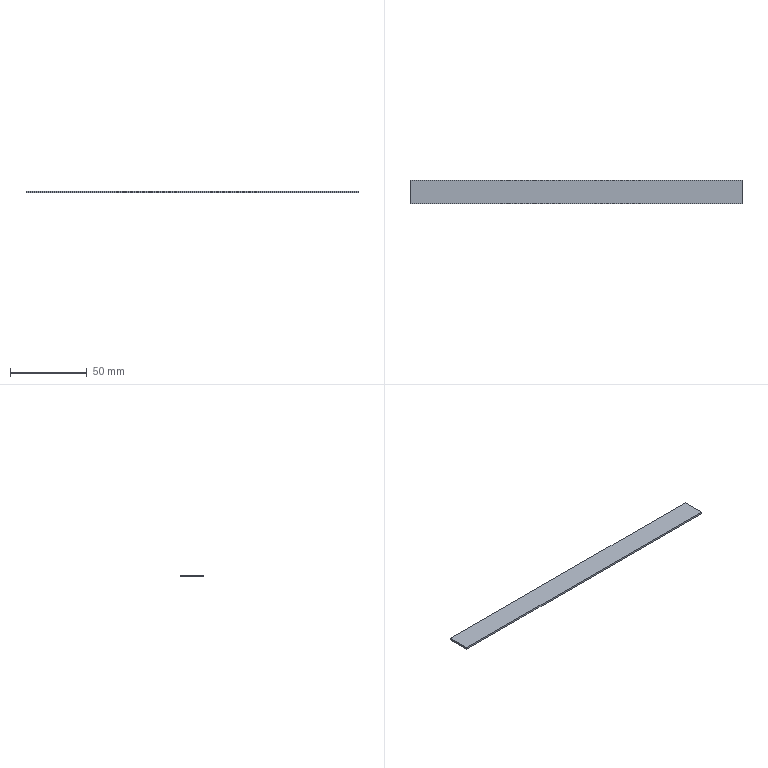Part | STEP file | gslz 2016.10.28-13_id1166_x_t | 1 solid | 6 faces | box 216.271 x 15 x 1.25 mm | volume 4055 mm3 | plane 6
STEP:
#1=CARTESIAN_POINT('',(0.,0.,0.));
#2=DIRECTION('',(0.,0.,1.));
#3=DIRECTION('',(1.,0.,0.));
#4=AXIS2_PLACEMENT_3D('',#1,#2,#3);
#5=CARTESIAN_POINT('',(-722.345,74.496,0.));
#6=VERTEX_POINT('',#5);
#7=CARTESIAN_POINT('',(-722.345,59.496,0.));
#8=VERTEX_POINT('',#7);
#9=CARTESIAN_POINT('',(-722.345,-271.75,0.));
#10=DIRECTION('',(0.,-1.,0.));
#11=VECTOR('',#10,1.);
#12=LINE('',#9,#11);
#13=CARTESIAN_POINT('',(-506.075,-394.584,0.));
#14=DIRECTION('',(0.,0.,-1.));
#15=DIRECTION('',(-1.,0.,0.));
#16=AXIS2_PLACEMENT_3D('',#13,#14,#15);
#17=PLANE('',#16);
#18=CARTESIAN_POINT('',(216.271,122.834));
#19=DIRECTION('',(0.,-1.));
#20=VECTOR('',#19,1.);
#21=LINE('',#18,#20);
#22=(GEOMETRIC_REPRESENTATION_CONTEXT(2)PARAMETRIC_REPRESENTATION_CONTEXT()REPRESENTATION_CONTEXT('',''));
#23=DEFINITIONAL_REPRESENTATION('',(#21),#22);
#24=PCURVE('',#17,#23);
#25=CARTESIAN_POINT('',(-722.345,-271.75,-0.75));
#26=DIRECTION('',(-1.,0.,0.));
#27=DIRECTION('',(0.,-1.,0.));
#28=AXIS2_PLACEMENT_3D('',#25,#26,#27);
#29=PLANE('',#28);
#30=CARTESIAN_POINT('',(0.,0.75));
#31=DIRECTION('',(1.,0.));
#32=VECTOR('',#31,1.);
#33=LINE('',#30,#32);
#34=(GEOMETRIC_REPRESENTATION_CONTEXT(2)PARAMETRIC_REPRESENTATION_CONTEXT()REPRESENTATION_CONTEXT('',''));
#35=DEFINITIONAL_REPRESENTATION('',(#33),#34);
#36=PCURVE('',#29,#35);
#37=SURFACE_CURVE('',#12,(#24,#36),.PCURVE_S1.);
#38=EDGE_CURVE('',#6,#8,#37,.T.);
#39=ORIENTED_EDGE('',*,*,#38,.F.);
#40=CARTESIAN_POINT('',(-506.075,74.496,0.));
#41=VERTEX_POINT('',#40);
#42=CARTESIAN_POINT('',(-506.075,74.496,0.));
#43=DIRECTION('',(-1.,0.,0.));
#44=VECTOR('',#43,1.);
#45=LINE('',#42,#44);
#46=CARTESIAN_POINT('',(0.,469.08));
#47=DIRECTION('',(1.,0.));
#48=VECTOR('',#47,1.);
#49=LINE('',#46,#48);
#50=(GEOMETRIC_REPRESENTATION_CONTEXT(2)PARAMETRIC_REPRESENTATION_CONTEXT()REPRESENTATION_CONTEXT('',''));
#51=DEFINITIONAL_REPRESENTATION('',(#49),#50);
#52=PCURVE('',#17,#51);
#53=CARTESIAN_POINT('',(-506.075,74.496,1.25));
#54=DIRECTION('',(0.,-1.,0.));
#55=DIRECTION('',(0.,0.,-1.));
#56=AXIS2_PLACEMENT_3D('',#53,#54,#55);
#57=PLANE('',#56);
#58=CARTESIAN_POINT('',(1.25,0.));
#59=DIRECTION('',(0.,-1.));
#60=VECTOR('',#59,1.);
#61=LINE('',#58,#60);
#62=(GEOMETRIC_REPRESENTATION_CONTEXT(2)PARAMETRIC_REPRESENTATION_CONTEXT()REPRESENTATION_CONTEXT('',''));
#63=DEFINITIONAL_REPRESENTATION('',(#61),#62);
#64=PCURVE('',#57,#63);
#65=SURFACE_CURVE('',#45,(#52,#64),.PCURVE_S1.);
#66=EDGE_CURVE('',#41,#6,#65,.T.);
#67=ORIENTED_EDGE('',*,*,#66,.F.);
#68=CARTESIAN_POINT('',(-506.075,59.496,0.));
#69=VERTEX_POINT('',#68);
#70=CARTESIAN_POINT('',(-506.075,-394.584,0.));
#71=DIRECTION('',(0.,-1.,0.));
#72=VECTOR('',#71,1.);
#73=LINE('',#70,#72);
#74=CARTESIAN_POINT('',(0.,0.));
#75=DIRECTION('',(0.,-1.));
#76=VECTOR('',#75,1.);
#77=LINE('',#74,#76);
#78=(GEOMETRIC_REPRESENTATION_CONTEXT(2)PARAMETRIC_REPRESENTATION_CONTEXT()REPRESENTATION_CONTEXT('',''));
#79=DEFINITIONAL_REPRESENTATION('',(#77),#78);
#80=PCURVE('',#17,#79);
#81=CARTESIAN_POINT('',(-506.075,-394.584,1.25));
#82=DIRECTION('',(-1.,0.,0.));
#83=DIRECTION('',(0.,-1.,0.));
#84=AXIS2_PLACEMENT_3D('',#81,#82,#83);
#85=PLANE('',#84);
#86=CARTESIAN_POINT('',(0.,-1.25));
#87=DIRECTION('',(1.,0.));
#88=VECTOR('',#87,1.);
#89=LINE('',#86,#88);
#90=(GEOMETRIC_REPRESENTATION_CONTEXT(2)PARAMETRIC_REPRESENTATION_CONTEXT()REPRESENTATION_CONTEXT('',''));
#91=DEFINITIONAL_REPRESENTATION('',(#89),#90);
#92=PCURVE('',#85,#91);
#93=SURFACE_CURVE('',#73,(#80,#92),.PCURVE_S1.);
#94=EDGE_CURVE('',#41,#69,#93,.T.);
#95=ORIENTED_EDGE('',*,*,#94,.T.);
#96=CARTESIAN_POINT('',(-506.075,59.496,0.));
#97=DIRECTION('',(-1.,0.,0.));
#98=VECTOR('',#97,1.);
#99=LINE('',#96,#98);
#100=CARTESIAN_POINT('',(0.,454.08));
#101=DIRECTION('',(1.,0.));
#102=VECTOR('',#101,1.);
#103=LINE('',#100,#102);
#104=(GEOMETRIC_REPRESENTATION_CONTEXT(2)PARAMETRIC_REPRESENTATION_CONTEXT()REPRESENTATION_CONTEXT('',''));
#105=DEFINITIONAL_REPRESENTATION('',(#103),#104);
#106=PCURVE('',#17,#105);
#107=CARTESIAN_POINT('',(-506.075,59.496,1.25));
#108=DIRECTION('',(0.,-1.,0.));
#109=DIRECTION('',(0.,0.,-1.));
#110=AXIS2_PLACEMENT_3D('',#107,#108,#109);
#111=PLANE('',#110);
#112=CARTESIAN_POINT('',(1.25,0.));
#113=DIRECTION('',(0.,-1.));
#114=VECTOR('',#113,1.);
#115=LINE('',#112,#114);
#116=(GEOMETRIC_REPRESENTATION_CONTEXT(2)PARAMETRIC_REPRESENTATION_CONTEXT()REPRESENTATION_CONTEXT('',''));
#117=DEFINITIONAL_REPRESENTATION('',(#115),#116);
#118=PCURVE('',#111,#117);
#119=SURFACE_CURVE('',#99,(#106,#118),.PCURVE_S1.);
#120=EDGE_CURVE('',#69,#8,#119,.T.);
#121=ORIENTED_EDGE('',*,*,#120,.T.);
#122=EDGE_LOOP('',(#39,#67,#95,#121));
#123=FACE_BOUND('',#122,.T.);
#124=ADVANCED_FACE('',(#123),#17,.T.);
#125=CARTESIAN_POINT('',(-722.345,59.496,1.25));
#126=VERTEX_POINT('',#125);
#127=CARTESIAN_POINT('',(-722.345,59.496,-0.75));
#128=DIRECTION('',(0.,0.,1.));
#129=VECTOR('',#128,1.);
#130=LINE('',#127,#129);
#131=CARTESIAN_POINT('',(2.,-216.271));
#132=DIRECTION('',(-1.,0.));
#133=VECTOR('',#132,1.);
#134=LINE('',#131,#133);
#135=(GEOMETRIC_REPRESENTATION_CONTEXT(2)PARAMETRIC_REPRESENTATION_CONTEXT()REPRESENTATION_CONTEXT('',''));
#136=DEFINITIONAL_REPRESENTATION('',(#134),#135);
#137=PCURVE('',#111,#136);
#138=CARTESIAN_POINT('',(-331.246,0.));
#139=DIRECTION('',(0.,1.));
#140=VECTOR('',#139,1.);
#141=LINE('',#138,#140);
#142=(GEOMETRIC_REPRESENTATION_CONTEXT(2)PARAMETRIC_REPRESENTATION_CONTEXT()REPRESENTATION_CONTEXT('',''));
#143=DEFINITIONAL_REPRESENTATION('',(#141),#142);
#144=PCURVE('',#29,#143);
#145=SURFACE_CURVE('',#130,(#137,#144),.PCURVE_S1.);
#146=EDGE_CURVE('',#8,#126,#145,.T.);
#147=ORIENTED_EDGE('',*,*,#146,.F.);
#148=ORIENTED_EDGE('',*,*,#120,.F.);
#149=CARTESIAN_POINT('',(-506.075,59.496,1.25));
#150=VERTEX_POINT('',#149);
#151=CARTESIAN_POINT('',(-506.075,59.496,1.25));
#152=DIRECTION('',(0.,0.,1.));
#153=VECTOR('',#152,1.);
#154=LINE('',#151,#153);
#155=CARTESIAN_POINT('',(0.,0.));
#156=DIRECTION('',(-1.,0.));
#157=VECTOR('',#156,1.);
#158=LINE('',#155,#157);
#159=(GEOMETRIC_REPRESENTATION_CONTEXT(2)PARAMETRIC_REPRESENTATION_CONTEXT()REPRESENTATION_CONTEXT('',''));
#160=DEFINITIONAL_REPRESENTATION('',(#158),#159);
#161=PCURVE('',#111,#160);
#162=CARTESIAN_POINT('',(-454.08,0.));
#163=DIRECTION('',(0.,1.));
#164=VECTOR('',#163,1.);
#165=LINE('',#162,#164);
#166=(GEOMETRIC_REPRESENTATION_CONTEXT(2)PARAMETRIC_REPRESENTATION_CONTEXT()REPRESENTATION_CONTEXT('',''));
#167=DEFINITIONAL_REPRESENTATION('',(#165),#166);
#168=PCURVE('',#85,#167);
#169=SURFACE_CURVE('',#154,(#161,#168),.PCURVE_S1.);
#170=EDGE_CURVE('',#69,#150,#169,.T.);
#171=ORIENTED_EDGE('',*,*,#170,.T.);
#172=CARTESIAN_POINT('',(-506.075,59.496,1.25));
#173=DIRECTION('',(-1.,0.,0.));
#174=VECTOR('',#173,1.);
#175=LINE('',#172,#174);
#176=CARTESIAN_POINT('',(0.,0.));
#177=DIRECTION('',(0.,-1.));
#178=VECTOR('',#177,1.);
#179=LINE('',#176,#178);
#180=(GEOMETRIC_REPRESENTATION_CONTEXT(2)PARAMETRIC_REPRESENTATION_CONTEXT()REPRESENTATION_CONTEXT('',''));
#181=DEFINITIONAL_REPRESENTATION('',(#179),#180);
#182=PCURVE('',#111,#181);
#183=CARTESIAN_POINT('',(-506.075,-394.584,1.25));
#184=DIRECTION('',(0.,0.,-1.));
#185=DIRECTION('',(-1.,0.,0.));
#186=AXIS2_PLACEMENT_3D('',#183,#184,#185);
#187=PLANE('',#186);
#188=CARTESIAN_POINT('',(0.,454.08));
#189=DIRECTION('',(1.,0.));
#190=VECTOR('',#189,1.);
#191=LINE('',#188,#190);
#192=(GEOMETRIC_REPRESENTATION_CONTEXT(2)PARAMETRIC_REPRESENTATION_CONTEXT()REPRESENTATION_CONTEXT('',''));
#193=DEFINITIONAL_REPRESENTATION('',(#191),#192);
#194=PCURVE('',#187,#193);
#195=SURFACE_CURVE('',#175,(#182,#194),.PCURVE_S1.);
#196=EDGE_CURVE('',#150,#126,#195,.T.);
#197=ORIENTED_EDGE('',*,*,#196,.T.);
#198=EDGE_LOOP('',(#147,#148,#171,#197));
#199=FACE_BOUND('',#198,.T.);
#200=ADVANCED_FACE('',(#199),#111,.T.);
#201=CARTESIAN_POINT('',(-722.345,74.496,1.25));
#202=VERTEX_POINT('',#201);
#203=CARTESIAN_POINT('',(-722.345,-271.75,1.25));
#204=DIRECTION('',(0.,-1.,0.));
#205=VECTOR('',#204,1.);
#206=LINE('',#203,#205);
#207=CARTESIAN_POINT('',(216.271,122.834));
#208=DIRECTION('',(0.,-1.));
#209=VECTOR('',#208,1.);
#210=LINE('',#207,#209);
#211=(GEOMETRIC_REPRESENTATION_CONTEXT(2)PARAMETRIC_REPRESENTATION_CONTEXT()REPRESENTATION_CONTEXT('',''));
#212=DEFINITIONAL_REPRESENTATION('',(#210),#211);
#213=PCURVE('',#187,#212);
#214=CARTESIAN_POINT('',(0.,2.));
#215=DIRECTION('',(1.,0.));
#216=VECTOR('',#215,1.);
#217=LINE('',#214,#216);
#218=(GEOMETRIC_REPRESENTATION_CONTEXT(2)PARAMETRIC_REPRESENTATION_CONTEXT()REPRESENTATION_CONTEXT('',''));
#219=DEFINITIONAL_REPRESENTATION('',(#217),#218);
#220=PCURVE('',#29,#219);
#221=SURFACE_CURVE('',#206,(#213,#220),.PCURVE_S1.);
#222=EDGE_CURVE('',#202,#126,#221,.T.);
#223=ORIENTED_EDGE('',*,*,#222,.T.);
#224=ORIENTED_EDGE('',*,*,#196,.F.);
#225=CARTESIAN_POINT('',(-506.075,74.496,1.25));
#226=VERTEX_POINT('',#225);
#227=CARTESIAN_POINT('',(-506.075,-394.584,1.25));
#228=DIRECTION('',(0.,-1.,0.));
#229=VECTOR('',#228,1.);
#230=LINE('',#227,#229);
#231=CARTESIAN_POINT('',(0.,0.));
#232=DIRECTION('',(0.,-1.));
#233=VECTOR('',#232,1.);
#234=LINE('',#231,#233);
#235=(GEOMETRIC_REPRESENTATION_CONTEXT(2)PARAMETRIC_REPRESENTATION_CONTEXT()REPRESENTATION_CONTEXT('',''));
#236=DEFINITIONAL_REPRESENTATION('',(#234),#235);
#237=PCURVE('',#187,#236);
#238=CARTESIAN_POINT('',(0.,0.));
#239=DIRECTION('',(1.,0.));
#240=VECTOR('',#239,1.);
#241=LINE('',#238,#240);
#242=(GEOMETRIC_REPRESENTATION_CONTEXT(2)PARAMETRIC_REPRESENTATION_CONTEXT()REPRESENTATION_CONTEXT('',''));
#243=DEFINITIONAL_REPRESENTATION('',(#241),#242);
#244=PCURVE('',#85,#243);
#245=SURFACE_CURVE('',#230,(#237,#244),.PCURVE_S1.);
#246=EDGE_CURVE('',#226,#150,#245,.T.);
#247=ORIENTED_EDGE('',*,*,#246,.F.);
#248=CARTESIAN_POINT('',(-506.075,74.496,1.25));
#249=DIRECTION('',(-1.,0.,0.));
#250=VECTOR('',#249,1.);
#251=LINE('',#248,#250);
#252=CARTESIAN_POINT('',(0.,469.08));
#253=DIRECTION('',(1.,0.));
#254=VECTOR('',#253,1.);
#255=LINE('',#252,#254);
#256=(GEOMETRIC_REPRESENTATION_CONTEXT(2)PARAMETRIC_REPRESENTATION_CONTEXT()REPRESENTATION_CONTEXT('',''));
#257=DEFINITIONAL_REPRESENTATION('',(#255),#256);
#258=PCURVE('',#187,#257);
#259=CARTESIAN_POINT('',(0.,0.));
#260=DIRECTION('',(0.,-1.));
#261=VECTOR('',#260,1.);
#262=LINE('',#259,#261);
#263=(GEOMETRIC_REPRESENTATION_CONTEXT(2)PARAMETRIC_REPRESENTATION_CONTEXT()REPRESENTATION_CONTEXT('',''));
#264=DEFINITIONAL_REPRESENTATION('',(#262),#263);
#265=PCURVE('',#57,#264);
#266=SURFACE_CURVE('',#251,(#258,#265),.PCURVE_S1.);
#267=EDGE_CURVE('',#226,#202,#266,.T.);
#268=ORIENTED_EDGE('',*,*,#267,.T.);
#269=EDGE_LOOP('',(#223,#224,#247,#268));
#270=FACE_BOUND('',#269,.T.);
#271=ADVANCED_FACE('',(#270),#187,.F.);
#272=CARTESIAN_POINT('',(-722.345,74.496,-0.75));
#273=DIRECTION('',(0.,0.,1.));
#274=VECTOR('',#273,1.);
#275=LINE('',#272,#274);
#276=CARTESIAN_POINT('',(2.,-216.271));
#277=DIRECTION('',(-1.,0.));
#278=VECTOR('',#277,1.);
#279=LINE('',#276,#278);
#280=(GEOMETRIC_REPRESENTATION_CONTEXT(2)PARAMETRIC_REPRESENTATION_CONTEXT()REPRESENTATION_CONTEXT('',''));
#281=DEFINITIONAL_REPRESENTATION('',(#279),#280);
#282=PCURVE('',#57,#281);
#283=CARTESIAN_POINT('',(-346.246,0.));
#284=DIRECTION('',(0.,1.));
#285=VECTOR('',#284,1.);
#286=LINE('',#283,#285);
#287=(GEOMETRIC_REPRESENTATION_CONTEXT(2)PARAMETRIC_REPRESENTATION_CONTEXT()REPRESENTATION_CONTEXT('',''));
#288=DEFINITIONAL_REPRESENTATION('',(#286),#287);
#289=PCURVE('',#29,#288);
#290=SURFACE_CURVE('',#275,(#282,#289),.PCURVE_S1.);
#291=EDGE_CURVE('',#6,#202,#290,.T.);
#292=ORIENTED_EDGE('',*,*,#291,.T.);
#293=ORIENTED_EDGE('',*,*,#267,.F.);
#294=CARTESIAN_POINT('',(-506.075,74.496,1.25));
#295=DIRECTION('',(0.,0.,1.));
#296=VECTOR('',#295,1.);
#297=LINE('',#294,#296);
#298=CARTESIAN_POINT('',(0.,0.));
#299=DIRECTION('',(-1.,0.));
#300=VECTOR('',#299,1.);
#301=LINE('',#298,#300);
#302=(GEOMETRIC_REPRESENTATION_CONTEXT(2)PARAMETRIC_REPRESENTATION_CONTEXT()REPRESENTATION_CONTEXT('',''));
#303=DEFINITIONAL_REPRESENTATION('',(#301),#302);
#304=PCURVE('',#57,#303);
#305=CARTESIAN_POINT('',(-469.08,0.));
#306=DIRECTION('',(0.,1.));
#307=VECTOR('',#306,1.);
#308=LINE('',#305,#307);
#309=(GEOMETRIC_REPRESENTATION_CONTEXT(2)PARAMETRIC_REPRESENTATION_CONTEXT()REPRESENTATION_CONTEXT('',''));
#310=DEFINITIONAL_REPRESENTATION('',(#308),#309);
#311=PCURVE('',#85,#310);
#312=SURFACE_CURVE('',#297,(#304,#311),.PCURVE_S1.);
#313=EDGE_CURVE('',#41,#226,#312,.T.);
#314=ORIENTED_EDGE('',*,*,#313,.F.);
#315=ORIENTED_EDGE('',*,*,#66,.T.);
#316=EDGE_LOOP('',(#292,#293,#314,#315));
#317=FACE_BOUND('',#316,.T.);
#318=ADVANCED_FACE('',(#317),#57,.F.);
#319=ORIENTED_EDGE('',*,*,#94,.F.);
#320=ORIENTED_EDGE('',*,*,#313,.T.);
#321=ORIENTED_EDGE('',*,*,#246,.T.);
#322=ORIENTED_EDGE('',*,*,#170,.F.);
#323=EDGE_LOOP('',(#319,#320,#321,#322));
#324=FACE_BOUND('',#323,.T.);
#325=ADVANCED_FACE('',(#324),#85,.F.);
#326=ORIENTED_EDGE('',*,*,#38,.T.);
#327=ORIENTED_EDGE('',*,*,#146,.T.);
#328=ORIENTED_EDGE('',*,*,#222,.F.);
#329=ORIENTED_EDGE('',*,*,#291,.F.);
#330=EDGE_LOOP('',(#326,#327,#328,#329));
#331=FACE_BOUND('',#330,.T.);
#332=ADVANCED_FACE('',(#331),#29,.T.);
#333=CLOSED_SHELL('',(#124,#200,#271,#318,#325,#332));
#334=MANIFOLD_SOLID_BREP('',#333);
#335=(LENGTH_UNIT()NAMED_UNIT(*)SI_UNIT(.MILLI.,.METRE.));
#336=UNCERTAINTY_MEASURE_WITH_UNIT(LENGTH_MEASURE(0.0000001),#335,'','');
#337=(NAMED_UNIT(*)PLANE_ANGLE_UNIT()SI_UNIT($,.RADIAN.));
#338=(NAMED_UNIT(*)SI_UNIT($,.STERADIAN.)SOLID_ANGLE_UNIT());
#339=(GEOMETRIC_REPRESENTATION_CONTEXT(3)GLOBAL_UNCERTAINTY_ASSIGNED_CONTEXT((#336))GLOBAL_UNIT_ASSIGNED_CONTEXT((#335,#337,#338))REPRESENTATION_CONTEXT('',''));
#340=ADVANCED_BREP_SHAPE_REPRESENTATION('',(#4,#334),#339);